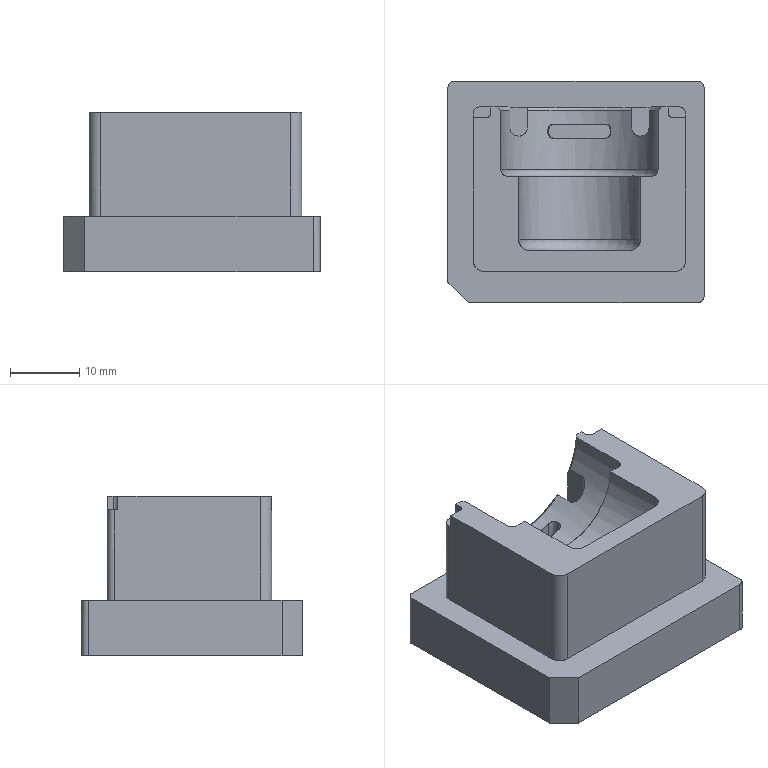NC program | PowerMill | posted with a generic post | part box 37 x 32 x 23 mm
Lines 1 to 1008 of 253511:
%
O0001
N104 ( POWERMILL CB  : 2026004.0)
N105 ( POST VER      : 2026.0.0.5161)
N106 ( OPTION FILE   : FANUC)
N107 ( OUTPUT WORKPLANE : WORLD)
N108 (  )
N109 ( TOOL LIST )
N110 (---------------------------------------)
N111 ( NO. | ID        | DIA.| TIP RAD|LENGTH)
N112 (---------------------------------------)
N113 (    1|D10C_1_1_1 |10.0 |  0.0   |78.44 )
N114 (   15|D3C_1_1    | 3.0 |  0.0   |66.32 )
N115 (   26|D1.5C_1_1  | 1.5 |  0.0   |68.34 )
N116 (    3|D10_1_1_1  |10.0 |  0.0   |78.16 )
N117 (   22|R1.5_1_1   | 3.0 |  1.5   | 67.4 )
N118 (    6|R0.5_1_1   | 1.0 |  0.5   |66.36 )
N119 (   20|D1.5_1_1   | 1.5 |  0.0   |68.46 )
N120 (    8|D1_1_1     | 1.0 |  0.0   |57.32 )
N121 (   13|TEXT_D4_1_1| 4.0 |  0.3   |70.28 )
N122 (---------------------------------------)
N123 (  )
N124 ( NUMBER OF TOOLPATHS: 15.0 )
N125 ( ESTIMATED PROGRAM DURATION: 0 HOURS 27 MIN 5 SEC)
N126 (  )
N127 G00 G21 G80 G40 G17
N128 G90
N129 G54
N130 G53 Z0.0
N131 (---------------)
N132 ( START TOOLPATH : 精公开粗01-扫面平行-D10C )
N133 (---------------)
N134 ( TOOL NO.    :1 )
N135 ( TOOL TYPE   : ENDMILL)
N136 ( TOOL ID     : D10C_1_1_1)
N137 ( TOOL DIA    : 10.0 LENGTH 78.44)
N138 T1
N139 M6
N140 S8000 M03
N141 G00 G90 X0.0 Y0.0
N142 G43 Z10.2 H1
N143
N144 G05 P10000 R4
N145 X26.28 Y18.78
N146 Z1.13
N147 G01 Z-0.07 F6000.0
N148 X21.28 F10000.0
N149 X-21.28
N150 Y13.4143
N151 X21.28
N152 Y8.0486
N153 X-21.28
N154 Y2.6829
N155 X21.28
N156 Y-2.6829
N157 X-21.28
N158 Y-8.0486
N159 X21.28
N160 Y-13.4143
N161 X-21.28
N162 Y-18.78
N163 X21.28
N164 X26.28
N165 G00 Z10.2
N166 G05 P0
N167 (---------------)
N168 ( END TOOLPATH : 精公开粗01-扫面平行-D10C )
N169 (---------------)
N170 ( START TOOLPATH : 精公开粗01-外形偏置-D10C )
N171 (---------------)
N172 G00 X0.4975 Y0.3775 Z9.88
N173 G05 P10000 R4
N174 X5.245 Y-24.554
N175 Z0.6948
N176 G01 Z-0.5052 F6000.0
N177 Y-24.0265 F10000.0
N178 G03 X0.4975 Y-19.279 I-4.7475 J0.0
N179 G01 X-21.639
N180 G02 X-22.639 Y-18.279 I0.0 J1.0
N181 G01 Y19.034
N182 G02 X-21.639 Y20.034 I1.0 J0.0
N183 G01 X22.634
N184 G02 X23.634 Y19.034 I0.0 J-1.0
N185 G01 Y-18.279
N186 G02 X22.634 Y-19.279 I-1.0 J0.0
N187 G01 X0.4975
N188 Y-16.7799
N189 X-13.0375
N190 X-13.8109 Y-16.7514
N191 X-14.5843 Y-16.6509
N192 X-15.3577 Y-16.4494
N193 X-16.1312 Y-16.1482
N194 X-16.9046 Y-15.7339
N195 X-17.678 Y-15.1629
N196 X-18.4514 Y-14.4051
N197 X-19.0936 Y-13.5442
N198 X-19.5077 Y-12.7708
N199 X-19.8085 Y-11.9973
N200 X-19.9983 Y-11.2802
N201 X-20.1102 Y-10.4505
N202 X-20.1385 Y-9.677
N203 Y10.432
N204 X-20.1144 Y11.2055
N205 X-19.9983 Y11.9096
N206 X-19.7237 Y12.7523
N207 X-19.3192 Y13.5258
N208 X-18.7224 Y14.2992
N209 X-18.4514 Y14.5698
N210 X-17.8192 Y15.0726
N211 X-16.9046 Y15.5682
N212 X-16.3245 Y15.7671
N213 X-16.2352 Y15.808
N214 X-16.1555 Y15.8655
N215 X-15.3577 Y16.5708
N216 X-14.5843 Y17.0228
N217 X-13.8109 Y17.3186
N218 X-13.0375 Y17.4851
N219 X-12.264 Y17.5344
N220 X-11.4906
N221 X-10.7172 Y17.4972
N222 X-10.1235 Y17.3929
N223 X-9.1703 Y17.069
N224 X-8.3969 Y16.6393
N225 X-7.6235 Y16.0066
N226 X-6.7297 Y15.0726
N227 X-6.2098 Y14.2992
N228 X-5.8616 Y13.5258
N229 X-5.6504 Y12.7523
N230 X-5.5592 Y11.9789
N231 X-5.5548 Y11.2055
N232 X-5.5543 Y7.0086
N233 G03 X-5.324 Y6.5877 I0.5 J0.0001
N234 G01 X-5.2885 Y6.5649
N235 X-4.5298 Y5.9351
N236 X-4.3913 Y5.7915
N237 X-3.7979 Y5.0181
N238 X-3.3959 Y4.2446
N239 X-3.14 Y3.4712
N240 X-3.0089 Y2.6978
N241 X-2.9858 Y1.9244
N242 X-2.9857 Y-2.72
N243 G03 X-2.4857 Y-3.22 I0.5 J0.0
N244 G01 X3.4815
N245 G03 X3.9815 Y-2.72 I0.0 J0.5
N246 G01 X3.9817 Y1.9244
N247 X4.0048 Y2.6978
N248 X4.1359 Y3.4712
N249 X4.3918 Y4.2446
N250 X4.7513 Y4.949
N251 X5.3872 Y5.7915
N252 X5.5248 Y5.9343
N253 X6.2982 Y6.5742
N254 X6.3193 Y6.5877
N255 G03 X6.5504 Y7.0092 I-0.2689 J0.4215
N256 G01 X6.5506 Y11.2055
N257 X6.5555 Y11.9789
N258 X6.5606 Y12.0224
N259 X1.5113 Y12.4765
N260 X1.4983 Y12.3327
N261 X1.3664 Y9.9945
N262 G02 X-0.374 Y10.0077 I-0.8699 J0.0473
N263 G01 X-0.4213 Y11.215
N264 X-0.4824 Y12.1301
N265 X-0.5936 Y13.0405
N266 X-0.6507 Y13.4206
N267 G02 X0.2338 Y14.4209 I0.8615 J0.1294
N268 G01 X0.7836 Y14.4063
N269 G02 X1.6018 Y13.4833 I-0.0223 J-0.8439
N270 G01 X1.5113 Y12.4765
N271 X6.5606 Y12.0224
N272 X6.6463 Y12.7523
N273 X6.8575 Y13.5258
N274 X7.0716 Y14.038
N275 X7.2057 Y14.2992
N276 X7.7256 Y15.0726
N277 X8.6185 Y16.0057
N278 X9.363 Y16.6195
N279 X10.1653 Y17.0686
N280 X10.9388 Y17.3461
N281 X11.7122 Y17.4971
N282 X12.4856 Y17.5344
N283 X13.259
N284 X14.0325 Y17.4852
N285 X14.8059 Y17.3189
N286 X15.5793 Y17.0232
N287 X16.3527 Y16.5715
N288 X17.1501 Y15.8665
N289 X17.2296 Y15.8091
N290 X17.3187 Y15.7683
N291 X17.8996 Y15.5685
N292 X18.673 Y15.1655
N293 X19.4464 Y14.5706
N294 X19.7183 Y14.2992
N295 X20.2199 Y13.6708
N296 X20.7195 Y12.7523
N297 X20.9774 Y11.9789
N298 X21.1102 Y11.2055
N299 X21.1344 Y10.432
N300 Y-9.677
N301 X21.106 Y-10.4505
N302 X21.0057 Y-11.2239
N303 X20.8044 Y-11.9973
N304 X20.5035 Y-12.7708
N305 X20.0894 Y-13.5442
N306 X19.5188 Y-14.3176
N307 X18.7618 Y-15.091
N308 X17.8996 Y-15.7345
N309 X17.1262 Y-16.1486
N310 X16.3527 Y-16.4496
N311 X15.6435 Y-16.6379
N312 X14.8059 Y-16.7515
N313 X14.0325 Y-16.7799
N314 X0.4975
N315 Y-19.279
N316 G00 Z3.3096
N317 G01 X5.245 Y-24.554
N318 G00 Z0.3096
N319 G01 Z-0.8904 F6000.0
N320 Y-24.0265 F10000.0
N321 G03 X0.4975 Y-19.279 I-4.7475 J0.0
N322 G01 X-21.639
N323 G02 X-22.639 Y-18.279 I0.0 J1.0
N324 G01 Y19.034
N325 G02 X-21.639 Y20.034 I1.0 J0.0
N326 G01 X22.634
N327 G02 X23.634 Y19.034 I0.0 J-1.0
N328 G01 Y-18.279
N329 G02 X22.634 Y-19.279 I-1.0 J0.0
N330 G01 X0.4975
N331 Y-16.7799
N332 X-13.0375
N333 X-13.8109 Y-16.7514
N334 X-14.5843 Y-16.6509
N335 X-15.3577 Y-16.4494
N336 X-16.1312 Y-16.1482
N337 X-16.9046 Y-15.7339
N338 X-17.678 Y-15.1629
N339 X-18.4514 Y-14.4051
N340 X-19.0936 Y-13.5442
N341 X-19.5077 Y-12.7708
N342 X-19.8085 Y-11.9973
N343 X-19.9983 Y-11.2802
N344 X-20.1102 Y-10.4505
N345 X-20.1385 Y-9.677
N346 Y10.432
N347 X-20.1144 Y11.2055
N348 X-19.9983 Y11.9097
N349 X-19.7237 Y12.7523
N350 X-19.3192 Y13.5258
N351 X-18.7224 Y14.2992
N352 X-18.4514 Y14.5698
N353 X-17.8192 Y15.0726
N354 X-16.9046 Y15.5682
N355 X-16.3245 Y15.7671
N356 X-16.2352 Y15.808
N357 X-16.1555 Y15.8655
N358 X-15.3577 Y16.5708
N359 X-14.5843 Y17.0228
N360 X-13.8109 Y17.3187
N361 X-13.0375 Y17.4851
N362 X-12.264 Y17.5344
N363 X-11.4906
N364 X-10.7172 Y17.5011
N365 X-10.0979 Y17.3929
N366 X-9.1703 Y17.0809
N367 X-8.3969 Y16.6563
N368 X-7.6235 Y16.0316
N369 X-6.7034 Y15.0726
N370 X-6.1835 Y14.2992
N371 X-5.8353 Y13.5258
N372 X-5.6297 Y12.7729
N373 X-0.622 Y13.3853
N374 X-0.6312 Y13.4603
N375 G02 X0.2237 Y14.4068 I0.838 J0.1025
N376 G01 X0.8028 Y14.3953
N377 G02 X1.6174 Y13.4401 I-0.0168 J-0.8393
N378 G01 X1.5428 Y12.9049
N379 X1.4456 Y12.0291
N380 X1.3975 Y11.1491
N381 X1.3687 Y10.0633
N382 G02 X-0.3726 Y10.0495 I-0.8709 J0.0231
N383 G01 X-0.4215 Y11.2014
N384 X-0.4732 Y12.0322
N385 X-0.5579 Y12.8604
N386 X-0.622 Y13.3853
N387 X-5.6297 Y12.7729
N388 X-5.6241 Y12.7523
N389 X-5.5323 Y11.9789
N390 X-5.5284 Y11.2055
N391 X-5.5276 Y7.0127
N392 G03 X-5.2976 Y6.5919 I0.5 J0.0001
N393 G01 X-5.2554 Y6.5649
N394 X-4.5298 Y5.968
N395 X-4.3583 Y5.7915
N396 X-3.7649 Y5.0181
N397 X-3.3628 Y4.2446
N398 X-3.107 Y3.4712
N399 X-2.9829 Y2.7676
N400 X-2.9528 Y1.9244
N401 Y-2.7197
N402 G03 X-2.4528 Y-3.2197 I0.5 J0.0
N403 G01 X3.4485 Y-3.22
N404 G03 X3.9485 Y-2.7199 I0.0 J0.5
N405 G01 X3.9483 Y1.9244
N406 X3.9717 Y2.6978
N407 X4.1028 Y3.4712
N408 X4.3587 Y4.2446
N409 X4.7513 Y5.0028
N410 X5.3542 Y5.7915
N411 X5.5248 Y5.9671
N412 X6.2982 Y6.5965
N413 G03 X6.5234 Y7.0142 I-0.2748 J0.4178
N414 G01 X6.5242 Y11.2055
N415 X6.5292 Y11.9789
N416 X6.6199 Y12.7523
N417 X6.8312 Y13.5258
N418 X7.1794 Y14.2992
N419 X7.6992 Y15.0726
N420 X8.6185 Y16.0308
N421 X9.3372 Y16.6195
N422 X10.1653 Y17.0804
N423 X10.9388 Y17.3539
N424 X11.7122 Y17.501
N425 X12.4856 Y17.5344
N426 X13.259
N427 X14.0325 Y17.4852
N428 X14.8059 Y17.3189
N429 X15.5793 Y17.0232
N430 X16.3527 Y16.5715
N431 X17.1501 Y15.8665
N432 X17.2296 Y15.8091
N433 X17.3187 Y15.7683
N434 X17.8996 Y15.5685
N435 X18.673 Y15.1655
N436 X19.4464 Y14.5706
N437 X19.7184 Y14.2992
N438 X20.2199 Y13.6708
N439 X20.7196 Y12.7523
N440 X20.9774 Y11.9789
N441 X21.1103 Y11.2055
N442 X21.1344 Y10.432
N443 Y-9.677
N444 X21.106 Y-10.4505
N445 X21.0057 Y-11.2239
N446 X20.8044 Y-11.9973
N447 X20.5035 Y-12.7708
N448 X20.0894 Y-13.5442
N449 X19.5188 Y-14.3176
N450 X18.7618 Y-15.091
N451 X17.8996 Y-15.7345
N452 X17.1262 Y-16.1486
N453 X16.3527 Y-16.4496
N454 X15.6435 Y-16.6379
N455 X14.8059 Y-16.7515
N456 X14.0325 Y-16.7799
N457 X0.4975
N458 Y-19.279
N459 G00 Z2.9244
N460 G01 X5.245 Y-24.554
N461 G00 Z-0.0756
N462 G01 Z-1.2756 F6000.0
N463 Y-24.0265 F10000.0
N464 G03 X0.4975 Y-19.279 I-4.7475 J0.0
N465 G01 X-21.639
N466 G02 X-22.639 Y-18.279 I0.0 J1.0
N467 G01 Y19.034
N468 G02 X-21.639 Y20.034 I1.0 J0.0
N469 G01 X22.634
N470 G02 X23.634 Y19.034 I0.0 J-1.0
N471 G01 Y-18.279
N472 G02 X22.634 Y-19.279 I-1.0 J0.0
N473 G01 X0.4975
N474 Y-16.7799
N475 X-13.0375
N476 X-13.8109 Y-16.7514
N477 X-14.5843 Y-16.6509
N478 X-15.3577 Y-16.4494
N479 X-16.1312 Y-16.1483
N480 X-16.9046 Y-15.7339
N481 X-17.678 Y-15.1629
N482 X-18.4514 Y-14.4051
N483 X-19.0936 Y-13.5442
N484 X-19.5077 Y-12.7708
N485 X-19.8085 Y-11.9973
N486 X-19.9983 Y-11.2802
N487 X-20.1102 Y-10.4505
N488 X-20.1385 Y-9.677
N489 Y10.432
N490 X-20.1144 Y11.2055
N491 X-19.9983 Y11.9097
N492 X-19.7237 Y12.7523
N493 X-19.3193 Y13.5258
N494 X-18.7224 Y14.2992
N495 X-18.4514 Y14.5698
N496 X-17.8192 Y15.0726
N497 X-16.9046 Y15.5683
N498 X-16.3245 Y15.7671
N499 X-16.2352 Y15.808
N500 X-16.1555 Y15.8655
N501 X-15.3577 Y16.5709
N502 X-14.5843 Y17.0228
N503 X-13.8109 Y17.3187
N504 X-13.0375 Y17.4851
N505 X-12.264 Y17.5344
N506 X-12.2613
N507 X-11.4906
N508 X-10.8608 Y17.5072
N509 X-10.7172 Y17.5045
N510 X-10.0664 Y17.3929
N511 X-9.1703 Y17.0945
N512 X-8.3969 Y16.6775
N513 X-7.6235 Y16.0627
N514 X-6.6718 Y15.0726
N515 X-6.1531 Y14.2992
N516 X-5.8051 Y13.5258
N517 X-5.5928 Y12.7523
N518 X-5.5031 Y11.9789
N519 X-5.4978 Y11.2055
N520 X-5.5001 Y7.025
N521 G03 X-5.2683 Y6.6028 I0.4999 J-0.0002
N522 G01 X-5.2088 Y6.5649
N523 X-4.5298 Y6.0145
N524 X-4.3118 Y5.7915
N525 X-3.7563 Y5.0774
N526 X-3.3152 Y4.2446
N527 X-3.0603 Y3.4712
N528 X-2.9282 Y2.6978
N529 X-2.9096 Y1.9244
N530 Y-2.7194
N531 G03 X-2.4097 Y-3.2194 I0.5 J0.0
N532 G01 X3.4047 Y-3.22
N533 G03 X3.9048 Y-2.72 I0.0001 J0.5
N534 G01 X3.9055 Y1.9244
N535 X3.9248 Y2.6978
N536 X4.0562 Y3.4712
N537 X4.3119 Y4.2446
N538 X4.7131 Y5.0181
N539 X5.3071 Y5.7915
N540 X5.5248 Y6.0135
N541 X6.205 Y6.5649
N542 X6.2634 Y6.602
N543 G03 X6.4951 Y7.0238 I-0.2683 J0.4219
N544 G01 X6.4965 Y11.9789
N545 X6.5203 Y12.1795
N546 X1.0845 Y12.9557
N547 G02 X-0.1095 Y12.9658 I-0.5963 J0.0851
N548 G01 X-0.1914 Y13.6188
N549 G02 X0.3217 Y14.1953 I0.5087 J0.0638
N550 G01 X0.6745 Y14.1922
N551 G02 X1.1775 Y13.6071 I-0.0045 J-0.5126
N552 G01 X1.0845 Y12.9557
N553 X6.5203 Y12.1795
N554 X6.5885 Y12.7523
N555 X6.7997 Y13.5258
N556 X7.0716 Y14.1559
N557 X7.668 Y15.0726
N558 X7.8451 Y15.2802
N559 X8.6185 Y16.0619
N560 X9.306 Y16.6195
N561 X10.1653 Y17.0942
N562 X10.9388 Y17.3622
N563 X11.7122 Y17.5044
N564 X12.4856 Y17.5344
N565 X13.259
N566 X14.0325 Y17.4852
N567 X14.8059 Y17.319
N568 X15.5793 Y17.0232
N569 X16.3527 Y16.5715
N570 X17.1501 Y15.8665
N571 X17.2296 Y15.8091
N572 X17.3188 Y15.7682
N573 X17.8996 Y15.5685
N574 X18.673 Y15.1655
N575 X19.4464 Y14.5707
N576 X19.7184 Y14.2992
N577 X20.2199 Y13.6708
N578 X20.7196 Y12.7523
N579 X20.9774 Y11.9789
N580 X21.1103 Y11.2055
N581 X21.1344 Y10.432
N582 Y-9.677
N583 X21.1061 Y-10.4505
N584 X21.0057 Y-11.2239
N585 X20.8044 Y-11.9973
N586 X20.5035 Y-12.7708
N587 X20.0894 Y-13.5442
N588 X19.5188 Y-14.3176
N589 X18.7618 Y-15.091
N590 X17.8996 Y-15.7345
N591 X17.1262 Y-16.1486
N592 X16.3527 Y-16.4496
N593 X15.6435 Y-16.6379
N594 X14.8059 Y-16.7515
N595 X14.0325 Y-16.7799
N596 X0.4975
N597 Y-19.279
N598 G00 Z2.5392
N599 G01 X5.245 Y-24.554
N600 G00 Z-0.4608
N601 G01 Z-1.6608 F6000.0
N602 Y-24.0265 F10000.0
N603 G03 X0.4975 Y-19.279 I-4.7475 J0.0
N604 G01 X-21.639
N605 G02 X-22.639 Y-18.279 I0.0 J1.0
N606 G01 Y19.034
N607 G02 X-21.639 Y20.034 I1.0 J0.0
N608 G01 X22.634
N609 G02 X23.634 Y19.034 I0.0 J-1.0
N610 G01 Y-18.279
N611 G02 X22.634 Y-19.279 I-1.0 J0.0
N612 G01 X0.4975
N613 Y-16.7799
N614 X-13.0375
N615 X-13.8109 Y-16.7514
N616 X-14.5843 Y-16.6509
N617 X-15.3577 Y-16.4494
N618 X-16.1312 Y-16.1483
N619 X-16.9046 Y-15.7339
N620 X-17.678 Y-15.1629
N621 X-18.4514 Y-14.4051
N622 X-19.0936 Y-13.5442
N623 X-19.5077 Y-12.7708
N624 X-19.8085 Y-11.9973
N625 X-19.9983 Y-11.2802
N626 X-20.1102 Y-10.4505
N627 X-20.1385 Y-9.677
N628 Y10.432
N629 X-20.1144 Y11.2055
N630 X-19.9983 Y11.9097
N631 X-19.7237 Y12.7523
N632 X-19.3193 Y13.5258
N633 X-18.7225 Y14.2992
N634 X-18.4514 Y14.5698
N635 X-17.8192 Y15.0726
N636 X-16.9046 Y15.5683
N637 X-16.3245 Y15.7671
N638 X-16.2351 Y15.808
N639 X-16.1555 Y15.8655
N640 X-15.3577 Y16.5709
N641 X-14.5843 Y17.0228
N642 X-13.8109 Y17.3187
N643 X-13.0375 Y17.4852
N644 X-12.264 Y17.5344
N645 X-12.2574 Y17.5343
N646 X-11.4906
N647 X-11.0415 Y17.515
N648 X-10.7172 Y17.5098
N649 X-10.0108 Y17.3929
N650 X-9.1703 Y17.1194
N651 X-8.3969 Y16.7141
N652 X-7.6235 Y16.1152
N653 X-6.8501 Y15.3469
N654 X-6.611 Y15.0726
N655 X-6.0911 Y14.2992
N656 X-5.7428 Y13.5258
N657 X-5.5309 Y12.7523
N658 X-5.4849 Y12.3574
N659 X-0.5225 Y13.4731
N660 G02 X0.6118 Y14.2425 I0.7185 J0.1615
N661 G01 X1.0198 Y13.9634
N662 G02 X1.0169 Y12.4245 I-0.5255 J-0.7685
N663 G02 X-0.4141 Y12.9907 I-0.5226 J0.7704
N664 G01 X-0.5225 Y13.4731
N665 X-5.4849 Y12.3574
N666 X-5.4408 Y11.9789
N667 X-5.4361 Y11.2055
N668 X-5.4359 Y7.031
N669 G03 X-5.2035 Y6.6087 I0.5 J0.0001
N670 G01 X-5.1343 Y6.5649
N671 X-4.5298 Y6.0828
N672 X-4.2371 Y5.7915
N673 X-3.6438 Y5.0181
N674 X-3.2418 Y4.2446
N675 X-2.9829 Y3.4577
N676 X-2.8547 Y2.6978
N677 X-2.8316 Y1.9244
N678 Y-2.7196
N679 G03 X-2.3406 Y-3.2195 I0.5 J0.0
N680 G01 X1.6915 Y-3.2199
N681 X3.3266 Y-3.22
N682 G03 X3.8267 Y-2.7201 I0.0001 J0.5
N683 G01 X3.8275 Y1.9244
N684 X3.8498 Y2.6978
N685 X3.9779 Y3.4545
N686 X4.237 Y4.2446
N687 X4.6398 Y5.0181
N688 X5.2326 Y5.7915
N689 X5.5248 Y6.0821
N690 X6.1307 Y6.5649
N691 X6.1998 Y6.6087
N692 G03 X6.432 Y7.0306 I-0.2678 J0.4223
N693 G01 X6.4357 Y11.9789
N694 X6.5267 Y12.7523
N695 X6.7379 Y13.5258
N696 X7.0858 Y14.2992
N697 X7.6071 Y15.0726
N698 X7.8451 Y15.3465
N699 X8.6185 Y16.1144
N700 X9.2497 Y16.6195
N701 X10.1653 Y17.119
N702 X10.9388 Y17.3767
N703 X11.7122 Y17.5097
N704 X11.9476 Y17.5135
N705 X12.4856 Y17.5344
N706 X13.2558
N707 X13.259
N708 X14.0325 Y17.4853
N709 X14.8059 Y17.319
N710 X15.5793 Y17.0232
N711 X16.3527 Y16.5715
N712 X17.1501 Y15.8665
N713 X17.2296 Y15.8091
N714 X17.3188 Y15.7682
N715 X17.8996 Y15.5686
N716 X18.673 Y15.1655
N717 X19.4464 Y14.5707
N718 X19.7184 Y14.2992
N719 X20.2199 Y13.6709
N720 X20.7196 Y12.7523
N721 X20.9775 Y11.9789
N722 X21.1103 Y11.2055
N723 X21.1344 Y10.432
N724 Y-9.677
N725 X21.1061 Y-10.4505
N726 X21.0057 Y-11.2239
N727 X20.8044 Y-11.9973
N728 X20.5035 Y-12.7708
N729 X20.0894 Y-13.5442
N730 X19.5188 Y-14.3176
N731 X18.7618 Y-15.091
N732 X17.8996 Y-15.7345
N733 X17.1262 Y-16.1486
N734 X16.3527 Y-16.4496
N735 X15.6435 Y-16.6379
N736 X14.8059 Y-16.7515
N737 X14.0325 Y-16.7799
N738 X0.4975
N739 Y-19.279
N740 G00 Z2.154
N741 G01 X5.245 Y-24.554
N742 G00 Z-0.846
N743 G01 Z-2.046 F6000.0
N744 Y-24.0265 F10000.0
N745 G03 X0.4975 Y-19.279 I-4.7475 J0.0
N746 G01 X-21.639
N747 G02 X-22.639 Y-18.279 I0.0 J1.0
N748 G01 Y19.034
N749 G02 X-21.639 Y20.034 I1.0 J0.0
N750 G01 X22.634
N751 G02 X23.634 Y19.034 I0.0 J-1.0
N752 G01 Y-18.279
N753 G02 X22.634 Y-19.279 I-1.0 J0.0
N754 G01 X0.4975
N755 Y-16.7799
N756 X-13.0375
N757 X-13.8109 Y-16.7514
N758 X-14.5843 Y-16.6509
N759 X-15.3577 Y-16.4494
N760 X-16.1312 Y-16.1483
N761 X-16.9046 Y-15.7339
N762 X-17.678 Y-15.1629
N763 X-18.4514 Y-14.4051
N764 X-19.0936 Y-13.5442
N765 X-19.5077 Y-12.7708
N766 X-19.8085 Y-11.9973
N767 X-19.9983 Y-11.2802
N768 X-20.1102 Y-10.4505
N769 X-20.1385 Y-9.677
N770 Y10.432
N771 X-20.1144 Y11.2055
N772 X-19.9983 Y11.9097
N773 X-19.7238 Y12.7523
N774 X-19.3193 Y13.5258
N775 X-18.7225 Y14.2992
N776 X-18.4514 Y14.5699
N777 X-17.8193 Y15.0726
N778 X-16.9046 Y15.5683
N779 X-16.3245 Y15.7671
N780 X-16.2351 Y15.808
N781 X-16.1555 Y15.8655
N782 X-15.3577 Y16.5709
N783 X-14.5843 Y17.0229
N784 X-13.8109 Y17.3187
N785 X-13.0375 Y17.4852
N786 X-12.264 Y17.5344
N787 X-12.2513 Y17.5343
N788 X-11.4906
N789 X-11.1852 Y17.5211
N790 X-10.7172 Y17.5153
N791 X-9.9503 Y17.3929
N792 X-9.1703 Y17.1442
N793 X-8.3969 Y16.751
N794 X-8.1938 Y16.6195
N795 X-7.6235 Y16.1709
N796 X-6.8501 Y15.4137
N797 X-6.5487 Y15.0726
N798 X-6.0766 Y14.3827
N799 X-5.6805 Y13.5258
N800 X-5.5564 Y13.074
N801 X-0.4928 Y13.6019
N802 G02 X-0.3971 Y14.025 I0.6732 J0.0702
N803 G02 X0.6451 Y14.1641 I0.5775 J-0.3529
N804 G01 X0.9034 Y13.9202
N805 G02 X0.2895 Y12.9156 I-0.4132 J-0.4374
N806 G01 X-0.0454 Y13.0341
N807 G02 X-0.4928 Y13.6019 I0.2258 J0.638
N808 G01 X-5.5564 Y13.074
N809 X-5.468 Y12.7523
N810 X-5.3785 Y11.9789
N811 X-5.3737 Y11.2055
N812 X-5.3723 Y7.0409
N813 G03 X-5.1395 Y6.6185 I0.5 J0.0002
N814 G01 X-5.0547 Y6.5649
N815 X-4.5298 Y6.1558
N816 X-4.1573 Y5.7915
N817 X-3.7563 Y5.3032
N818 X-3.5622 Y5.0181
N819 X-3.1602 Y4.2446
N820 X-2.9054 Y3.4712
N821 X-2.7739 Y2.6978
N822 X-2.7536 Y1.9244
N823 Y-2.7199
N824 G03 X-2.2726 Y-3.2195 I0.5 J0.0
N825 G01 X1.6915 Y-3.2199
N826 X2.9259 Y-3.22
N827 X3.2492
N828 G03 X3.7492 Y-2.72 I0.0 J0.5
N829 G01 X3.7495 Y1.9244
N830 X3.7701 Y2.6978
N831 X3.8999 Y3.4712
N832 X4.1573 Y4.2446
N833 X4.5581 Y5.0181
N834 X4.7513 Y5.3018
N835 X5.1531 Y5.7915
N836 X5.5248 Y6.155
N837 X6.0495 Y6.5649
N838 X6.135 Y6.6187
N839 G03 X6.3687 Y7.0415 I-0.2663 J0.4232
N840 G01 X6.3733 Y11.9789
N841 X6.4649 Y12.7523
N842 X6.6761 Y13.5258
N843 X7.0237 Y14.2992
N844 X7.5438 Y15.0726
N845 X7.8451 Y15.4128
N846 X8.6185 Y16.1702
N847 X9.1896 Y16.6195
N848 X9.3919 Y16.7502
N849 X10.1653 Y17.1438
N850 X10.9388 Y17.3911
N851 X11.7122 Y17.5153
N852 X12.1268 Y17.5204
N853 X12.4856 Y17.5343
N854 X13.2507
N855 X13.259 Y17.5344
N856 X14.0325 Y17.4853
N857 X14.8059 Y17.319
N858 X15.5793 Y17.0233
N859 X16.3527 Y16.5716
N860 X17.1501 Y15.8665
N861 X17.2296 Y15.8091
N862 X17.3188 Y15.7682
N863 X17.8996 Y15.5686
N864 X18.673 Y15.1655
N865 X19.4464 Y14.5707
N866 X19.7184 Y14.2992
N867 X20.2199 Y13.6709
N868 X20.7196 Y12.7523
N869 X20.9775 Y11.9789
N870 X21.1103 Y11.2055
N871 X21.1344 Y10.432
N872 Y-9.677
N873 X21.1061 Y-10.4505
N874 X21.0057 Y-11.2239
N875 X20.8044 Y-11.9973
N876 X20.5035 Y-12.7708
N877 X20.0894 Y-13.5442
N878 X19.5188 Y-14.3176
N879 X18.7618 Y-15.091
N880 X17.8996 Y-15.7345
N881 X17.1262 Y-16.1486
N882 X16.3527 Y-16.4496
N883 X15.6435 Y-16.6379
N884 X14.8059 Y-16.7515
N885 X14.0325 Y-16.7799
N886 X0.4975
N887 Y-19.279
N888 G00 Z1.7612
N889 G01 X5.245 Y-24.554
N890 G00 Z-1.2388
N891 G01 Z-2.4388 F6000.0
N892 Y-24.0265 F10000.0
N893 G03 X0.4975 Y-19.279 I-4.7475 J0.0
N894 G01 X-21.639
N895 G02 X-22.639 Y-18.279 I0.0 J1.0
N896 G01 Y19.034
N897 G02 X-21.639 Y20.034 I1.0 J0.0
N898 G01 X22.634
N899 G02 X23.634 Y19.034 I0.0 J-1.0
N900 G01 Y-18.279
N901 G02 X22.634 Y-19.279 I-1.0 J0.0
N902 G01 X0.4975
N903 Y-16.7799
N904 X-13.0375
N905 X-13.8109 Y-16.7514
N906 X-14.5843 Y-16.6509
N907 X-15.3577 Y-16.4494
N908 X-16.1312 Y-16.1483
N909 X-16.9046 Y-15.7339
N910 X-17.678 Y-15.1629
N911 X-18.4514 Y-14.4051
N912 X-19.0936 Y-13.5442
N913 X-19.5077 Y-12.7708
N914 X-19.8085 Y-11.9973
N915 X-19.9983 Y-11.2802
N916 X-20.1102 Y-10.4505
N917 X-20.1385 Y-9.677
N918 Y11.2055
N919 X-20.0892 Y11.9789
N920 X-19.9983 Y12.5707
N921 X-19.7114 Y13.5258
N922 X-19.3511 Y14.2992
N923 X-18.8441 Y15.0726
N924 X-18.4514 Y15.5364
N925 X-18.1419 Y15.846
N926 X-17.678 Y16.2389
N927 X-16.9046 Y16.7462
N928 X-16.1312 Y17.1068
N929 X-15.3577 Y17.3529
N930 X-14.5843 Y17.4849
N931 X-13.8109 Y17.5344
N932 X-12.3613 Y17.5282
N933 X-12.264 Y17.5344
N934 X-12.2513 Y17.5342
N935 X-11.4906
N936 X-11.2384 Y17.5234
N937 X-10.7172 Y17.5211
N938 X-9.9438 Y17.4101
N939 X-9.1703 Y17.1753
N940 X-8.3969 Y16.7978
N941 X-8.1159 Y16.6195
N942 X-7.6235 Y16.2404
N943 X-6.8501 Y15.4937
N944 X-6.4689 Y15.0726
N945 X-6.0766 Y14.5175
N946 X-5.9488 Y14.2992
N947 X-5.5995 Y13.5258
N948 X-5.3891 Y12.7523
N949 X-5.3032 Y12.0684
N950 X-5.2928 Y11.2055
N951 X-5.2933 Y10.6742
N952 X0.1985 Y10.6811
N953 X0.1968 Y12.0753
N954 X0.1859 Y12.4152
N955 X0.1539 Y12.7537
N956 X0.068 Y13.4377
N957 X0.0063 Y13.8197
N958 X-0.0821 Y14.1964
N959 X-0.1739 Y14.534
N960 X1.1702
N961 X1.0795 Y14.202
N962 X0.9858 Y13.8007
N963 X0.9225 Y13.3936
N964 X0.8317 Y12.6201
N965 X0.8037 Y12.3024
N966 X0.7942 Y11.9835
N967 X0.7919 Y9.2825
N968 X0.5562 Y9.0045
N969 X0.5269 Y8.9697
N970 X0.498 Y8.9346
N971 X0.4682 Y8.9707
N972 X0.438 Y9.0065
N973 X0.2003 Y9.2868
N974 X0.1985 Y10.6811
N975 X-5.2933 Y10.6742
N976 X-5.2969 Y7.0631
N977 G03 X-5.091 Y6.6583 I0.5 J-0.0005
N978 G01 X-4.5298 Y6.25
N979 X-4.047 Y5.7915
N980 X-3.7563 Y5.4488
N981 X-3.4532 Y5.0181
N982 X-3.0508 Y4.2446
N983 X-2.7948 Y3.4712
N984 X-2.6636 Y2.6978
N985 X-2.6405 Y1.9244
N986 Y-2.72
N987 G03 X-2.1601 Y-3.2196 I0.5 J0.0
N988 G01 X1.6915 Y-3.22
N989 X2.3611
N990 X3.1359
N991 G03 X3.6359 Y-2.72 I0.0 J0.5
N992 G01 X3.6361 Y1.9244
N993 X3.6595 Y2.6978
N994 X3.7907 Y3.4712
N995 X4.0467 Y4.2446
N996 X4.4488 Y5.0181
N997 X4.7513 Y5.4477
N998 X5.0428 Y5.7915
N999 X5.5248 Y6.2492
N1000 X5.9406 Y6.5649
N1001 X6.0555 Y6.6369
N1002 G03 X6.29 Y7.0608 I-0.2655 J0.4237
N1003 G01 X6.2882 Y11.2055
N1004 X6.2942 Y11.9789
N1005 X6.385 Y12.7523
N1006 X6.5963 Y13.5258
N1007 X6.9446 Y14.2992
N1008 X7.0716 Y14.516
N1009 X7.4647 Y15.0726
N1010 X7.8451 Y15.4936
N1011 X8.6185 Y16.2397
N1012 X9.1115 Y16.6195
N1013 X9.3919 Y16.7972
N1014 X10.1653 Y17.1749
N1015 X10.8676 Y17.3929
N1016 X11.7122 Y17.5211
N1017 X12.199 Y17.5232
N1018 X12.4856 Y17.5343
N1019 X13.2507
N1020 X13.259 Y17.5344
N1021 X13.357 Y17.5282
N1022 X14.8059 Y17.5344
N1023 X15.5793 Y17.485
N1024 X16.1772 Y17.3929
N1025 X17.1262 Y17.1072
N1026 X17.8996 Y16.7467
N1027 X18.673 Y16.2396
N1028 X19.1377 Y15.846
N1029 X19.4464 Y15.5373
N1030 X19.8399 Y15.0726
N1031 X20.347 Y14.2992
N1032 X20.7073 Y13.5258
N1033 X20.9531 Y12.7523
N1034 X21.085 Y11.9789
N1035 X21.1344 Y11.2055
N1036 Y-9.677
N1037 X21.1061 Y-10.4505
N1038 X21.0057 Y-11.2239
N1039 X20.8044 Y-11.9973
N1040 X20.5035 Y-12.7708
N1041 X20.0894 Y-13.5442
N1042 X19.5188 Y-14.3176
N1043 X18.7618 Y-15.091
N1044 X17.8996 Y-15.7345
N1045 X17.1262 Y-16.1486
N1046 X16.3527 Y-16.4497
N1047 X15.6435 Y-16.6379
N1048 X14.8059 Y-16.7515
N1049 X14.0325 Y-16.7799
N1050 X0.4975
N1051 Y-19.279
N1052 G00 Z1.3683
N1053 G01 X5.245 Y-24.554
N1054 G00 Z-1.6317
N1055 G01 Z-2.8317 F6000.0
N1056 Y-24.0265 F10000.0
N1057 G03 X0.4975 Y-19.279 I-4.7475 J0.0
N1058 G01 X-21.639
N1059 G02 X-22.639 Y-18.279 I0.0 J1.0
N1060 G01 Y19.034
N1061 G02 X-21.639 Y20.034 I1.0 J0.0
N1062 G01 X22.634
N1063 G02 X23.634 Y19.034 I0.0 J-1.0
N1064 G01 Y-18.279
N1065 G02 X22.634 Y-19.279 I-1.0 J0.0
N1066 G01 X0.4975
N1067 Y-16.7799
N1068 X-13.0375
N1069 X-13.8109 Y-16.7514
N1070 X-14.5843 Y-16.6509
N1071 X-15.3577 Y-16.4494
N1072 X-16.1312 Y-16.1483
N1073 X-16.9046 Y-15.7339
N1074 X-17.678 Y-15.1629
N1075 X-18.4514 Y-14.4051
N1076 X-19.0936 Y-13.5442
N1077 X-19.5077 Y-12.7708
N1078 X-19.8085 Y-11.9973
N1079 X-19.9983 Y-11.2802
N1080 X-20.1102 Y-10.4505
N1081 X-20.1385 Y-9.677
N1082 Y11.2055
N1083 X-20.0892 Y11.9789
N1084 X-19.9983 Y12.5707
N1085 X-19.7114 Y13.5258
N1086 X-19.3511 Y14.2992
N1087 X-18.8441 Y15.0726
N1088 X-18.4514 Y15.5364
N1089 X-18.1419 Y15.846
N1090 X-17.678 Y16.239
N1091 X-16.9046 Y16.7462
N1092 X-16.1312 Y17.1068
N1093 X-15.3577 Y17.3529
N1094 X-14.5843 Y17.4849
N1095 X-13.8109 Y17.5344
N1096 X-12.3192 Y17.5308
N1097 X-12.264 Y17.5343
N1098 X-12.2513 Y17.5342
N1099 X-11.4906
N1100 X-11.3588 Y17.5285
N1101 X-10.7172 Y17.527
N1102 X-9.9438 Y17.4294
N1103 X-9.1703 Y17.2106
N1104 X-8.3969 Y16.8525
N1105 X-8.0205 Y16.6195